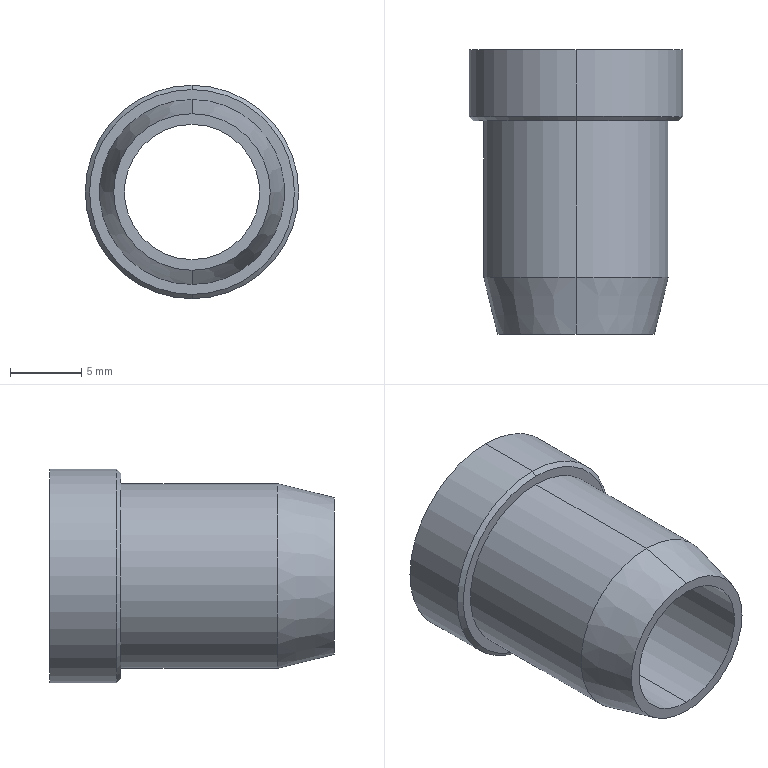Part | SolidWorks | features Chamfer 3, ICE 2, Extrusion 1 | 1 solid | 18 faces | box 15 x 20 x 15 mm | volume 1157 mm3 | cylinder 8 | cone 6 | plane 4 | commonest cylinder face diameters 9.5 x2 12 x2 13 x2 15 x2
STEP:
#1=CARTESIAN_POINT('',(0.,0.,-5.5));
#2=VERTEX_POINT('',#1);
#3=CARTESIAN_POINT('',(0.,0.,5.5));
#4=VERTEX_POINT('',#3);
#5=CARTESIAN_POINT('',(0.,0.,0.));
#6=DIRECTION('',(0.,-1.,0.));
#7=DIRECTION('',(0.,0.,1.));
#8=AXIS2_PLACEMENT_3D('',#5,#6,#7);
#9=CIRCLE('',#8,5.5);
#10=EDGE_CURVE('',#2,#4,#9,.T.);
#11=ORIENTED_EDGE('',*,*,#10,.F.);
#12=CARTESIAN_POINT('',(0.,4.,-6.5));
#13=VERTEX_POINT('',#12);
#14=CARTESIAN_POINT('',(0.,0.,-5.5));
#15=DIRECTION('',(0.,0.9701,-0.2425));
#16=VECTOR('',#15,1000.);
#17=LINE('',#14,#16);
#18=EDGE_CURVE('',#2,#13,#17,.T.);
#19=ORIENTED_EDGE('',*,*,#18,.T.);
#20=CARTESIAN_POINT('',(0.,4.,6.5));
#21=VERTEX_POINT('',#20);
#22=CARTESIAN_POINT('',(0.,4.,0.));
#23=DIRECTION('',(0.,1.,0.));
#24=DIRECTION('',(0.,0.,1.));
#25=AXIS2_PLACEMENT_3D('',#22,#23,#24);
#26=CIRCLE('',#25,6.5);
#27=EDGE_CURVE('',#21,#13,#26,.T.);
#28=ORIENTED_EDGE('',*,*,#27,.F.);
#29=CARTESIAN_POINT('',(0.,0.,5.5));
#30=DIRECTION('',(0.,0.9701,0.2425));
#31=VECTOR('',#30,1000.);
#32=LINE('',#29,#31);
#33=EDGE_CURVE('',#4,#21,#32,.T.);
#34=ORIENTED_EDGE('',*,*,#33,.F.);
#35=EDGE_LOOP('',(#11,#19,#28,#34));
#36=FACE_OUTER_BOUND('',#35,.T.);
#37=CARTESIAN_POINT('',(0.,0.,0.));
#38=DIRECTION('',(0.,1.,0.));
#39=DIRECTION('',(0.,0.,1.));
#40=AXIS2_PLACEMENT_3D('',#37,#38,#39);
#41=CONICAL_SURFACE('',#40,5.5,0.245);
#42=ADVANCED_FACE('',(#36),#41,.T.);
#43=CARTESIAN_POINT('',(0.,15.,-7.2));
#44=VERTEX_POINT('',#43);
#45=CARTESIAN_POINT('',(0.,15.,7.2));
#46=VERTEX_POINT('',#45);
#47=CARTESIAN_POINT('',(0.,15.,0.));
#48=DIRECTION('',(0.,-1.,0.));
#49=DIRECTION('',(0.,0.,-1.));
#50=AXIS2_PLACEMENT_3D('',#47,#48,#49);
#51=CIRCLE('',#50,7.2);
#52=EDGE_CURVE('',#44,#46,#51,.T.);
#53=ORIENTED_EDGE('',*,*,#52,.F.);
#54=CARTESIAN_POINT('',(0.,15.3,-7.5));
#55=VERTEX_POINT('',#54);
#56=CARTESIAN_POINT('',(0.,15.,-7.2));
#57=DIRECTION('',(0.,0.7071,-0.7071));
#58=VECTOR('',#57,1000.);
#59=LINE('',#56,#58);
#60=EDGE_CURVE('',#44,#55,#59,.T.);
#61=ORIENTED_EDGE('',*,*,#60,.T.);
#62=CARTESIAN_POINT('',(0.,15.3,7.5));
#63=VERTEX_POINT('',#62);
#64=CARTESIAN_POINT('',(0.,15.3,0.));
#65=DIRECTION('',(0.,1.,0.));
#66=DIRECTION('',(0.,0.,-1.));
#67=AXIS2_PLACEMENT_3D('',#64,#65,#66);
#68=CIRCLE('',#67,7.5);
#69=EDGE_CURVE('',#63,#55,#68,.T.);
#70=ORIENTED_EDGE('',*,*,#69,.F.);
#71=CARTESIAN_POINT('',(0.,15.,7.2));
#72=DIRECTION('',(0.,0.7071,0.7071));
#73=VECTOR('',#72,1000.);
#74=LINE('',#71,#73);
#75=EDGE_CURVE('',#46,#63,#74,.T.);
#76=ORIENTED_EDGE('',*,*,#75,.F.);
#77=EDGE_LOOP('',(#53,#61,#70,#76));
#78=FACE_OUTER_BOUND('',#77,.T.);
#79=CARTESIAN_POINT('',(0.,15.,0.));
#80=DIRECTION('',(0.,1.,0.));
#81=DIRECTION('',(0.,0.,1.));
#82=AXIS2_PLACEMENT_3D('',#79,#80,#81);
#83=CONICAL_SURFACE('',#82,7.2,0.7854);
#84=ADVANCED_FACE('',(#78),#83,.T.);
#85=CARTESIAN_POINT('',(0.,7.,-4.75));
#86=VERTEX_POINT('',#85);
#87=CARTESIAN_POINT('',(0.,7.,4.75));
#88=VERTEX_POINT('',#87);
#89=CARTESIAN_POINT('',(0.,7.,0.));
#90=DIRECTION('',(0.,1.,0.));
#91=DIRECTION('',(0.,0.,1.));
#92=AXIS2_PLACEMENT_3D('',#89,#90,#91);
#93=CIRCLE('',#92,4.75);
#94=EDGE_CURVE('',#86,#88,#93,.T.);
#95=ORIENTED_EDGE('',*,*,#94,.F.);
#96=CARTESIAN_POINT('',(0.,17.,-5.35));
#97=VERTEX_POINT('',#96);
#98=CARTESIAN_POINT('',(0.,7.,-4.75));
#99=DIRECTION('',(0.,0.9982,-0.05989));
#100=VECTOR('',#99,1000.);
#101=LINE('',#98,#100);
#102=EDGE_CURVE('',#86,#97,#101,.T.);
#103=ORIENTED_EDGE('',*,*,#102,.T.);
#104=CARTESIAN_POINT('',(0.,17.,5.35));
#105=VERTEX_POINT('',#104);
#106=CARTESIAN_POINT('',(0.,17.,0.));
#107=DIRECTION('',(0.,-1.,0.));
#108=DIRECTION('',(0.,0.,1.));
#109=AXIS2_PLACEMENT_3D('',#106,#107,#108);
#110=CIRCLE('',#109,5.35);
#111=EDGE_CURVE('',#105,#97,#110,.T.);
#112=ORIENTED_EDGE('',*,*,#111,.F.);
#113=CARTESIAN_POINT('',(0.,7.,4.75));
#114=DIRECTION('',(0.,0.9982,0.05989));
#115=VECTOR('',#114,1000.);
#116=LINE('',#113,#115);
#117=EDGE_CURVE('',#88,#105,#116,.T.);
#118=ORIENTED_EDGE('',*,*,#117,.F.);
#119=EDGE_LOOP('',(#95,#103,#112,#118));
#120=FACE_OUTER_BOUND('',#119,.T.);
#121=CARTESIAN_POINT('',(0.,7.,0.));
#122=DIRECTION('',(0.,1.,0.));
#123=DIRECTION('',(0.,0.,1.));
#124=AXIS2_PLACEMENT_3D('',#121,#122,#123);
#125=CONICAL_SURFACE('',#124,4.75,0.05993);
#126=ADVANCED_FACE('',(#120),#125,.F.);
#127=CARTESIAN_POINT('',(0.,15.,-6.5));
#128=VERTEX_POINT('',#127);
#129=CARTESIAN_POINT('',(0.,15.,6.5));
#130=VERTEX_POINT('',#129);
#131=CARTESIAN_POINT('',(0.,15.,0.));
#132=DIRECTION('',(0.,-1.,0.));
#133=DIRECTION('',(0.,0.,-1.));
#134=AXIS2_PLACEMENT_3D('',#131,#132,#133);
#135=CIRCLE('',#134,6.5);
#136=EDGE_CURVE('',#128,#130,#135,.T.);
#137=ORIENTED_EDGE('',*,*,#136,.T.);
#138=CARTESIAN_POINT('',(0.,15.,6.5));
#139=DIRECTION('',(0.,-1.,0.));
#140=VECTOR('',#139,1000.);
#141=LINE('',#138,#140);
#142=EDGE_CURVE('',#130,#21,#141,.T.);
#143=ORIENTED_EDGE('',*,*,#142,.T.);
#144=ORIENTED_EDGE('',*,*,#27,.T.);
#145=CARTESIAN_POINT('',(0.,15.,-6.5));
#146=DIRECTION('',(0.,-1.,0.));
#147=VECTOR('',#146,1000.);
#148=LINE('',#145,#147);
#149=EDGE_CURVE('',#128,#13,#148,.T.);
#150=ORIENTED_EDGE('',*,*,#149,.F.);
#151=EDGE_LOOP('',(#137,#143,#144,#150));
#152=FACE_OUTER_BOUND('',#151,.T.);
#153=CARTESIAN_POINT('',(0.,15.,0.));
#154=DIRECTION('',(0.,-1.,0.));
#155=DIRECTION('',(0.,0.,-1.));
#156=AXIS2_PLACEMENT_3D('',#153,#154,#155);
#157=CYLINDRICAL_SURFACE('',#156,6.5);
#158=ADVANCED_FACE('',(#152),#157,.T.);
#159=CARTESIAN_POINT('',(0.,17.,-6.));
#160=VERTEX_POINT('',#159);
#161=CARTESIAN_POINT('',(0.,17.,6.));
#162=VERTEX_POINT('',#161);
#163=CARTESIAN_POINT('',(0.,17.,0.));
#164=DIRECTION('',(0.,1.,0.));
#165=DIRECTION('',(0.,0.,1.));
#166=AXIS2_PLACEMENT_3D('',#163,#164,#165);
#167=CIRCLE('',#166,6.);
#168=EDGE_CURVE('',#160,#162,#167,.T.);
#169=ORIENTED_EDGE('',*,*,#168,.F.);
#170=CARTESIAN_POINT('',(0.,20.,-6.));
#171=VERTEX_POINT('',#170);
#172=CARTESIAN_POINT('',(0.,17.,-6.));
#173=DIRECTION('',(0.,1.,0.));
#174=VECTOR('',#173,1000.);
#175=LINE('',#172,#174);
#176=EDGE_CURVE('',#160,#171,#175,.T.);
#177=ORIENTED_EDGE('',*,*,#176,.T.);
#178=CARTESIAN_POINT('',(0.,20.,6.));
#179=VERTEX_POINT('',#178);
#180=CARTESIAN_POINT('',(0.,20.,0.));
#181=DIRECTION('',(0.,1.,0.));
#182=DIRECTION('',(0.,0.,1.));
#183=AXIS2_PLACEMENT_3D('',#180,#181,#182);
#184=CIRCLE('',#183,6.);
#185=EDGE_CURVE('',#171,#179,#184,.T.);
#186=ORIENTED_EDGE('',*,*,#185,.T.);
#187=CARTESIAN_POINT('',(0.,17.,6.));
#188=DIRECTION('',(0.,1.,0.));
#189=VECTOR('',#188,1000.);
#190=LINE('',#187,#189);
#191=EDGE_CURVE('',#162,#179,#190,.T.);
#192=ORIENTED_EDGE('',*,*,#191,.F.);
#193=EDGE_LOOP('',(#169,#177,#186,#192));
#194=FACE_OUTER_BOUND('',#193,.T.);
#195=CARTESIAN_POINT('',(0.,17.,0.));
#196=DIRECTION('',(0.,1.,0.));
#197=DIRECTION('',(0.,0.,1.));
#198=AXIS2_PLACEMENT_3D('',#195,#196,#197);
#199=CYLINDRICAL_SURFACE('',#198,6.);
#200=ADVANCED_FACE('',(#194),#199,.F.);
#201=ORIENTED_EDGE('',*,*,#94,.T.);
#202=CARTESIAN_POINT('',(0.,0.,4.75));
#203=VERTEX_POINT('',#202);
#204=CARTESIAN_POINT('',(0.,20.,4.75));
#205=DIRECTION('',(0.,-1.,0.));
#206=VECTOR('',#205,1000.);
#207=LINE('',#204,#206);
#208=EDGE_CURVE('',#88,#203,#207,.T.);
#209=ORIENTED_EDGE('',*,*,#208,.T.);
#210=CARTESIAN_POINT('',(0.,0.,-4.75));
#211=VERTEX_POINT('',#210);
#212=CARTESIAN_POINT('',(0.,0.,0.));
#213=DIRECTION('',(0.,1.,0.));
#214=DIRECTION('',(0.,0.,1.));
#215=AXIS2_PLACEMENT_3D('',#212,#213,#214);
#216=CIRCLE('',#215,4.75);
#217=EDGE_CURVE('',#211,#203,#216,.T.);
#218=ORIENTED_EDGE('',*,*,#217,.F.);
#219=CARTESIAN_POINT('',(0.,20.,-4.75));
#220=DIRECTION('',(0.,-1.,0.));
#221=VECTOR('',#220,1000.);
#222=LINE('',#219,#221);
#223=EDGE_CURVE('',#86,#211,#222,.T.);
#224=ORIENTED_EDGE('',*,*,#223,.F.);
#225=EDGE_LOOP('',(#201,#209,#218,#224));
#226=FACE_OUTER_BOUND('',#225,.T.);
#227=CARTESIAN_POINT('',(0.,20.,0.));
#228=DIRECTION('',(0.,-1.,0.));
#229=DIRECTION('',(0.,0.,-1.));
#230=AXIS2_PLACEMENT_3D('',#227,#228,#229);
#231=CYLINDRICAL_SURFACE('',#230,4.75);
#232=ADVANCED_FACE('',(#226),#231,.F.);
#233=CARTESIAN_POINT('',(0.,20.,7.5));
#234=VERTEX_POINT('',#233);
#235=CARTESIAN_POINT('',(0.,20.,-7.5));
#236=VERTEX_POINT('',#235);
#237=CARTESIAN_POINT('',(0.,20.,0.));
#238=DIRECTION('',(0.,1.,0.));
#239=DIRECTION('',(0.,0.,1.));
#240=AXIS2_PLACEMENT_3D('',#237,#238,#239);
#241=CIRCLE('',#240,7.5);
#242=EDGE_CURVE('',#234,#236,#241,.T.);
#243=ORIENTED_EDGE('',*,*,#242,.F.);
#244=CARTESIAN_POINT('',(0.,20.,7.5));
#245=DIRECTION('',(0.,-1.,0.));
#246=VECTOR('',#245,1000.);
#247=LINE('',#244,#246);
#248=EDGE_CURVE('',#234,#63,#247,.T.);
#249=ORIENTED_EDGE('',*,*,#248,.T.);
#250=ORIENTED_EDGE('',*,*,#69,.T.);
#251=CARTESIAN_POINT('',(0.,20.,-7.5));
#252=DIRECTION('',(0.,-1.,0.));
#253=VECTOR('',#252,1000.);
#254=LINE('',#251,#253);
#255=EDGE_CURVE('',#236,#55,#254,.T.);
#256=ORIENTED_EDGE('',*,*,#255,.F.);
#257=EDGE_LOOP('',(#243,#249,#250,#256));
#258=FACE_OUTER_BOUND('',#257,.T.);
#259=CARTESIAN_POINT('',(0.,20.,0.));
#260=DIRECTION('',(0.,-1.,0.));
#261=DIRECTION('',(0.,0.,-1.));
#262=AXIS2_PLACEMENT_3D('',#259,#260,#261);
#263=CYLINDRICAL_SURFACE('',#262,7.5);
#264=ADVANCED_FACE('',(#258),#263,.T.);
#265=CARTESIAN_POINT('',(0.,0.,0.));
#266=DIRECTION('',(0.,-1.,0.));
#267=DIRECTION('',(0.,0.,1.));
#268=AXIS2_PLACEMENT_3D('',#265,#266,#267);
#269=CIRCLE('',#268,5.5);
#270=EDGE_CURVE('',#4,#2,#269,.T.);
#271=ORIENTED_EDGE('',*,*,#270,.T.);
#272=ORIENTED_EDGE('',*,*,#10,.T.);
#273=EDGE_LOOP('',(#271,#272));
#274=FACE_OUTER_BOUND('',#273,.T.);
#275=ORIENTED_EDGE('',*,*,#217,.T.);
#276=CARTESIAN_POINT('',(0.,0.,0.));
#277=DIRECTION('',(0.,1.,0.));
#278=DIRECTION('',(0.,0.,1.));
#279=AXIS2_PLACEMENT_3D('',#276,#277,#278);
#280=CIRCLE('',#279,4.75);
#281=EDGE_CURVE('',#203,#211,#280,.T.);
#282=ORIENTED_EDGE('',*,*,#281,.T.);
#283=EDGE_LOOP('',(#275,#282));
#284=FACE_BOUND('',#283,.T.);
#285=CARTESIAN_POINT('',(0.,0.,0.));
#286=DIRECTION('',(0.,1.,0.));
#287=DIRECTION('',(0.,0.,1.));
#288=AXIS2_PLACEMENT_3D('',#285,#286,#287);
#289=PLANE('',#288);
#290=ADVANCED_FACE('',(#274,#284),#289,.F.);
#291=ORIENTED_EDGE('',*,*,#248,.F.);
#292=CARTESIAN_POINT('',(0.,20.,0.));
#293=DIRECTION('',(0.,1.,0.));
#294=DIRECTION('',(0.,0.,1.));
#295=AXIS2_PLACEMENT_3D('',#292,#293,#294);
#296=CIRCLE('',#295,7.5);
#297=EDGE_CURVE('',#236,#234,#296,.T.);
#298=ORIENTED_EDGE('',*,*,#297,.F.);
#299=ORIENTED_EDGE('',*,*,#255,.T.);
#300=CARTESIAN_POINT('',(0.,15.3,0.));
#301=DIRECTION('',(0.,1.,0.));
#302=DIRECTION('',(0.,0.,-1.));
#303=AXIS2_PLACEMENT_3D('',#300,#301,#302);
#304=CIRCLE('',#303,7.5);
#305=EDGE_CURVE('',#55,#63,#304,.T.);
#306=ORIENTED_EDGE('',*,*,#305,.T.);
#307=EDGE_LOOP('',(#291,#298,#299,#306));
#308=FACE_OUTER_BOUND('',#307,.T.);
#309=CARTESIAN_POINT('',(0.,20.,0.));
#310=DIRECTION('',(0.,-1.,0.));
#311=DIRECTION('',(0.,0.,-1.));
#312=AXIS2_PLACEMENT_3D('',#309,#310,#311);
#313=CYLINDRICAL_SURFACE('',#312,7.5);
#314=ADVANCED_FACE('',(#308),#313,.T.);
#315=ORIENTED_EDGE('',*,*,#208,.F.);
#316=CARTESIAN_POINT('',(0.,7.,0.));
#317=DIRECTION('',(0.,1.,0.));
#318=DIRECTION('',(0.,0.,1.));
#319=AXIS2_PLACEMENT_3D('',#316,#317,#318);
#320=CIRCLE('',#319,4.75);
#321=EDGE_CURVE('',#88,#86,#320,.T.);
#322=ORIENTED_EDGE('',*,*,#321,.T.);
#323=ORIENTED_EDGE('',*,*,#223,.T.);
#324=ORIENTED_EDGE('',*,*,#281,.F.);
#325=EDGE_LOOP('',(#315,#322,#323,#324));
#326=FACE_OUTER_BOUND('',#325,.T.);
#327=CARTESIAN_POINT('',(0.,20.,0.));
#328=DIRECTION('',(0.,-1.,0.));
#329=DIRECTION('',(0.,0.,-1.));
#330=AXIS2_PLACEMENT_3D('',#327,#328,#329);
#331=CYLINDRICAL_SURFACE('',#330,4.75);
#332=ADVANCED_FACE('',(#326),#331,.F.);
#333=CARTESIAN_POINT('',(0.,20.,0.));
#334=DIRECTION('',(0.,1.,0.));
#335=DIRECTION('',(0.,0.,1.));
#336=AXIS2_PLACEMENT_3D('',#333,#334,#335);
#337=CIRCLE('',#336,6.);
#338=EDGE_CURVE('',#179,#171,#337,.T.);
#339=ORIENTED_EDGE('',*,*,#338,.F.);
#340=ORIENTED_EDGE('',*,*,#185,.F.);
#341=EDGE_LOOP('',(#339,#340));
#342=FACE_BOUND('',#341,.T.);
#343=ORIENTED_EDGE('',*,*,#297,.T.);
#344=ORIENTED_EDGE('',*,*,#242,.T.);
#345=EDGE_LOOP('',(#343,#344));
#346=FACE_OUTER_BOUND('',#345,.T.);
#347=CARTESIAN_POINT('',(0.,20.,0.));
#348=DIRECTION('',(0.,1.,0.));
#349=DIRECTION('',(0.,0.,1.));
#350=AXIS2_PLACEMENT_3D('',#347,#348,#349);
#351=PLANE('',#350);
#352=ADVANCED_FACE('',(#342,#346),#351,.T.);
#353=ORIENTED_EDGE('',*,*,#176,.F.);
#354=CARTESIAN_POINT('',(0.,17.,0.));
#355=DIRECTION('',(0.,1.,0.));
#356=DIRECTION('',(0.,0.,1.));
#357=AXIS2_PLACEMENT_3D('',#354,#355,#356);
#358=CIRCLE('',#357,6.);
#359=EDGE_CURVE('',#162,#160,#358,.T.);
#360=ORIENTED_EDGE('',*,*,#359,.F.);
#361=ORIENTED_EDGE('',*,*,#191,.T.);
#362=ORIENTED_EDGE('',*,*,#338,.T.);
#363=EDGE_LOOP('',(#353,#360,#361,#362));
#364=FACE_OUTER_BOUND('',#363,.T.);
#365=CARTESIAN_POINT('',(0.,17.,0.));
#366=DIRECTION('',(0.,1.,0.));
#367=DIRECTION('',(0.,0.,1.));
#368=AXIS2_PLACEMENT_3D('',#365,#366,#367);
#369=CYLINDRICAL_SURFACE('',#368,6.);
#370=ADVANCED_FACE('',(#364),#369,.F.);
#371=ORIENTED_EDGE('',*,*,#111,.T.);
#372=CARTESIAN_POINT('',(0.,17.,0.));
#373=DIRECTION('',(0.,-1.,0.));
#374=DIRECTION('',(0.,0.,1.));
#375=AXIS2_PLACEMENT_3D('',#372,#373,#374);
#376=CIRCLE('',#375,5.35);
#377=EDGE_CURVE('',#97,#105,#376,.T.);
#378=ORIENTED_EDGE('',*,*,#377,.T.);
#379=EDGE_LOOP('',(#371,#378));
#380=FACE_BOUND('',#379,.T.);
#381=ORIENTED_EDGE('',*,*,#359,.T.);
#382=ORIENTED_EDGE('',*,*,#168,.T.);
#383=EDGE_LOOP('',(#381,#382));
#384=FACE_OUTER_BOUND('',#383,.T.);
#385=CARTESIAN_POINT('',(0.,17.,0.));
#386=DIRECTION('',(0.,1.,0.));
#387=DIRECTION('',(0.,0.,1.));
#388=AXIS2_PLACEMENT_3D('',#385,#386,#387);
#389=PLANE('',#388);
#390=ADVANCED_FACE('',(#380,#384),#389,.T.);
#391=CARTESIAN_POINT('',(0.,15.,0.));
#392=DIRECTION('',(0.,-1.,0.));
#393=DIRECTION('',(0.,0.,-1.));
#394=AXIS2_PLACEMENT_3D('',#391,#392,#393);
#395=CIRCLE('',#394,7.2);
#396=EDGE_CURVE('',#46,#44,#395,.T.);
#397=ORIENTED_EDGE('',*,*,#396,.T.);
#398=ORIENTED_EDGE('',*,*,#52,.T.);
#399=EDGE_LOOP('',(#397,#398));
#400=FACE_OUTER_BOUND('',#399,.T.);
#401=ORIENTED_EDGE('',*,*,#136,.F.);
#402=CARTESIAN_POINT('',(0.,15.,0.));
#403=DIRECTION('',(0.,-1.,0.));
#404=DIRECTION('',(0.,0.,-1.));
#405=AXIS2_PLACEMENT_3D('',#402,#403,#404);
#406=CIRCLE('',#405,6.5);
#407=EDGE_CURVE('',#130,#128,#406,.T.);
#408=ORIENTED_EDGE('',*,*,#407,.F.);
#409=EDGE_LOOP('',(#401,#408));
#410=FACE_BOUND('',#409,.T.);
#411=CARTESIAN_POINT('',(0.,15.,0.));
#412=DIRECTION('',(0.,-1.,0.));
#413=DIRECTION('',(0.,0.,-1.));
#414=AXIS2_PLACEMENT_3D('',#411,#412,#413);
#415=PLANE('',#414);
#416=ADVANCED_FACE('',(#400,#410),#415,.T.);
#417=ORIENTED_EDGE('',*,*,#142,.F.);
#418=ORIENTED_EDGE('',*,*,#407,.T.);
#419=ORIENTED_EDGE('',*,*,#149,.T.);
#420=CARTESIAN_POINT('',(0.,4.,0.));
#421=DIRECTION('',(0.,1.,0.));
#422=DIRECTION('',(0.,0.,1.));
#423=AXIS2_PLACEMENT_3D('',#420,#421,#422);
#424=CIRCLE('',#423,6.5);
#425=EDGE_CURVE('',#13,#21,#424,.T.);
#426=ORIENTED_EDGE('',*,*,#425,.T.);
#427=EDGE_LOOP('',(#417,#418,#419,#426));
#428=FACE_OUTER_BOUND('',#427,.T.);
#429=CARTESIAN_POINT('',(0.,15.,0.));
#430=DIRECTION('',(0.,-1.,0.));
#431=DIRECTION('',(0.,0.,-1.));
#432=AXIS2_PLACEMENT_3D('',#429,#430,#431);
#433=CYLINDRICAL_SURFACE('',#432,6.5);
#434=ADVANCED_FACE('',(#428),#433,.T.);
#435=ORIENTED_EDGE('',*,*,#102,.F.);
#436=ORIENTED_EDGE('',*,*,#321,.F.);
#437=ORIENTED_EDGE('',*,*,#117,.T.);
#438=ORIENTED_EDGE('',*,*,#377,.F.);
#439=EDGE_LOOP('',(#435,#436,#437,#438));
#440=FACE_OUTER_BOUND('',#439,.T.);
#441=CARTESIAN_POINT('',(0.,7.,0.));
#442=DIRECTION('',(0.,1.,0.));
#443=DIRECTION('',(0.,0.,1.));
#444=AXIS2_PLACEMENT_3D('',#441,#442,#443);
#445=CONICAL_SURFACE('',#444,4.75,0.05993);
#446=ADVANCED_FACE('',(#440),#445,.F.);
#447=ORIENTED_EDGE('',*,*,#60,.F.);
#448=ORIENTED_EDGE('',*,*,#396,.F.);
#449=ORIENTED_EDGE('',*,*,#75,.T.);
#450=ORIENTED_EDGE('',*,*,#305,.F.);
#451=EDGE_LOOP('',(#447,#448,#449,#450));
#452=FACE_OUTER_BOUND('',#451,.T.);
#453=CARTESIAN_POINT('',(0.,15.,0.));
#454=DIRECTION('',(0.,1.,0.));
#455=DIRECTION('',(0.,0.,1.));
#456=AXIS2_PLACEMENT_3D('',#453,#454,#455);
#457=CONICAL_SURFACE('',#456,7.2,0.7854);
#458=ADVANCED_FACE('',(#452),#457,.T.);
#459=ORIENTED_EDGE('',*,*,#18,.F.);
#460=ORIENTED_EDGE('',*,*,#270,.F.);
#461=ORIENTED_EDGE('',*,*,#33,.T.);
#462=ORIENTED_EDGE('',*,*,#425,.F.);
#463=EDGE_LOOP('',(#459,#460,#461,#462));
#464=FACE_OUTER_BOUND('',#463,.T.);
#465=CARTESIAN_POINT('',(0.,0.,0.));
#466=DIRECTION('',(0.,1.,0.));
#467=DIRECTION('',(0.,0.,1.));
#468=AXIS2_PLACEMENT_3D('',#465,#466,#467);
#469=CONICAL_SURFACE('',#468,5.5,0.245);
#470=ADVANCED_FACE('',(#464),#469,.T.);
#471=CLOSED_SHELL('',(#42,#84,#126,#158,#200,#232,#264,#290,#314,#332,#352,#370,#390,#416,#434,#446,#458,#470));
#472=MANIFOLD_SOLID_BREP('',#471);
#473=CARTESIAN_POINT('',(0.,0.,0.));
#474=DIRECTION('',(0.,0.,1.));
#475=DIRECTION('',(1.,0.,0.));
#476=AXIS2_PLACEMENT_3D('',#473,#474,#475);
#477=(LENGTH_UNIT()NAMED_UNIT(*)SI_UNIT(.MILLI.,.METRE.));
#478=UNCERTAINTY_MEASURE_WITH_UNIT(LENGTH_MEASURE(0.00001),#477,'','');
#479=(NAMED_UNIT(*)PLANE_ANGLE_UNIT()SI_UNIT($,.RADIAN.));
#480=(NAMED_UNIT(*)SI_UNIT($,.STERADIAN.)SOLID_ANGLE_UNIT());
#481=(GEOMETRIC_REPRESENTATION_CONTEXT(3)GLOBAL_UNCERTAINTY_ASSIGNED_CONTEXT((#478))GLOBAL_UNIT_ASSIGNED_CONTEXT((#477,#479,#480))REPRESENTATION_CONTEXT('',''));
#482=ADVANCED_BREP_SHAPE_REPRESENTATION('',(#472,#476),#481);